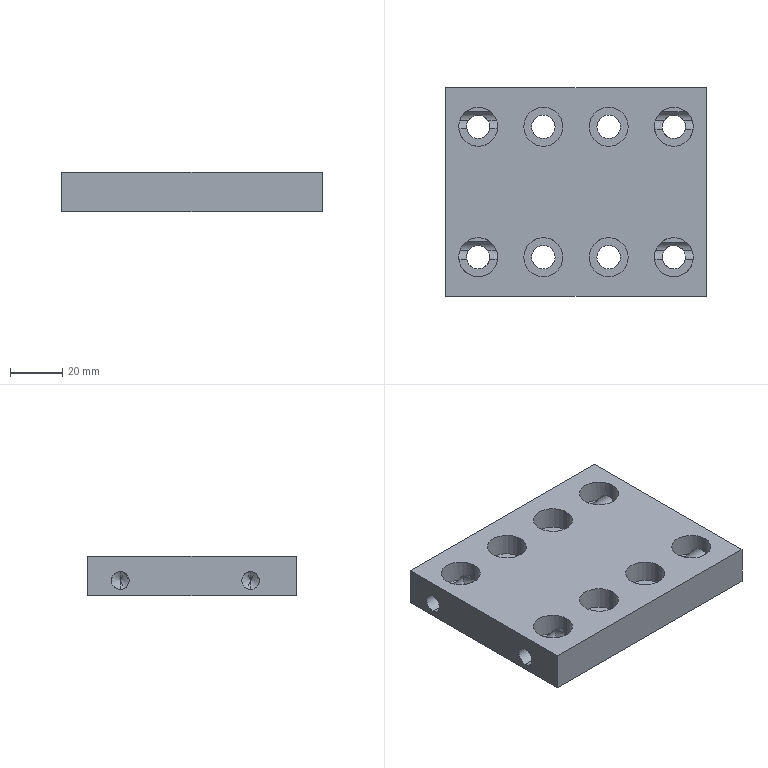Part | NX | features BREP 1 | 1 solid | 74 faces | box 100 x 80 x 15 mm | volume 102928 mm3 | cylinder 48 | plane 18 | cone 8 | commonest cylinder face diameters 6.8 x16 9 x16 15 x16